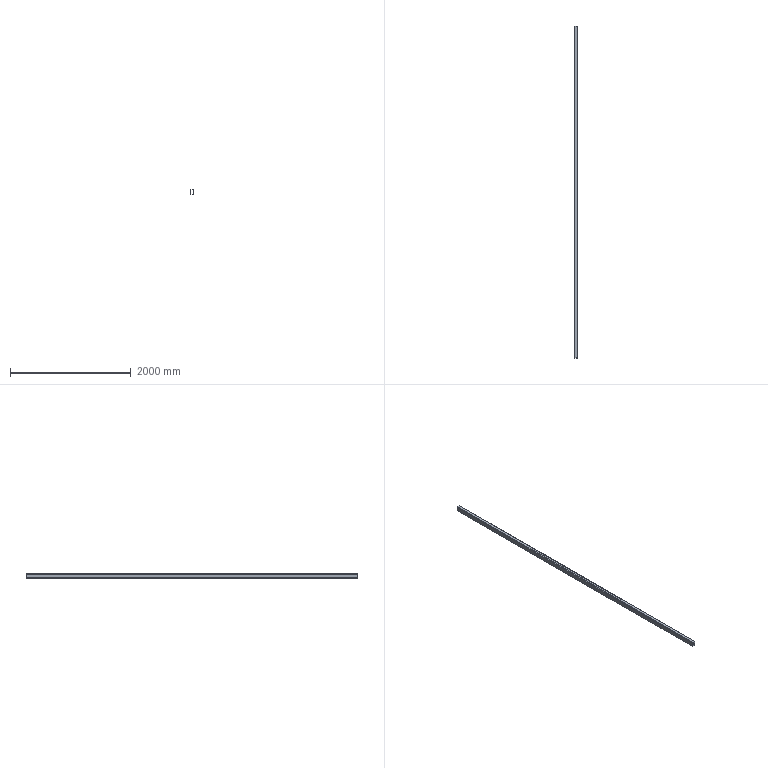Part | SolidWorks | features WeldMemberFeat 1, WeldmentFeature 1 | 1 solid | 18 faces | box 60 x 5500 x 80 mm | volume 6795907 mm3 | plane 10 | cylinder 8 | commonest cylinder face diameters 10 x4 20 x4
STEP:
#1=CARTESIAN_POINT('',(-30.,0.,30.));
#2=VERTEX_POINT('',#1);
#3=CARTESIAN_POINT('',(-20.,0.,40.));
#4=VERTEX_POINT('',#3);
#5=CARTESIAN_POINT('',(-20.,0.,30.));
#6=DIRECTION('',(0.,1.,0.));
#7=DIRECTION('',(0.,0.,1.));
#8=AXIS2_PLACEMENT_3D('',#5,#6,#7);
#9=CIRCLE('',#8,10.);
#10=EDGE_CURVE('',#2,#4,#9,.T.);
#11=ORIENTED_EDGE('',*,*,#10,.T.);
#12=CARTESIAN_POINT('',(-20.,5500.,40.));
#13=VERTEX_POINT('',#12);
#14=CARTESIAN_POINT('',(-20.,5500.,40.));
#15=DIRECTION('',(0.,-1.,0.));
#16=VECTOR('',#15,1000.);
#17=LINE('',#14,#16);
#18=EDGE_CURVE('',#13,#4,#17,.T.);
#19=ORIENTED_EDGE('',*,*,#18,.F.);
#20=CARTESIAN_POINT('',(-30.,5500.,30.));
#21=VERTEX_POINT('',#20);
#22=CARTESIAN_POINT('',(-20.,5500.,30.));
#23=DIRECTION('',(0.,1.,0.));
#24=DIRECTION('',(0.,0.,1.));
#25=AXIS2_PLACEMENT_3D('',#22,#23,#24);
#26=CIRCLE('',#25,10.);
#27=EDGE_CURVE('',#21,#13,#26,.T.);
#28=ORIENTED_EDGE('',*,*,#27,.F.);
#29=CARTESIAN_POINT('',(-30.,5500.,30.));
#30=DIRECTION('',(0.,-1.,0.));
#31=VECTOR('',#30,1000.);
#32=LINE('',#29,#31);
#33=EDGE_CURVE('',#21,#2,#32,.T.);
#34=ORIENTED_EDGE('',*,*,#33,.T.);
#35=EDGE_LOOP('',(#11,#19,#28,#34));
#36=FACE_OUTER_BOUND('',#35,.T.);
#37=CARTESIAN_POINT('',(-20.,5500.,30.));
#38=DIRECTION('',(0.,-1.,0.));
#39=DIRECTION('',(0.,0.,-1.));
#40=AXIS2_PLACEMENT_3D('',#37,#38,#39);
#41=CYLINDRICAL_SURFACE('',#40,10.);
#42=ADVANCED_FACE('',(#36),#41,.T.);
#43=CARTESIAN_POINT('',(20.,0.,40.));
#44=VERTEX_POINT('',#43);
#45=CARTESIAN_POINT('',(-20.,0.,40.));
#46=DIRECTION('',(1.,0.,0.));
#47=VECTOR('',#46,1000.);
#48=LINE('',#45,#47);
#49=EDGE_CURVE('',#4,#44,#48,.T.);
#50=ORIENTED_EDGE('',*,*,#49,.T.);
#51=CARTESIAN_POINT('',(20.,5500.,40.));
#52=VERTEX_POINT('',#51);
#53=CARTESIAN_POINT('',(20.,5500.,40.));
#54=DIRECTION('',(0.,-1.,0.));
#55=VECTOR('',#54,1000.);
#56=LINE('',#53,#55);
#57=EDGE_CURVE('',#52,#44,#56,.T.);
#58=ORIENTED_EDGE('',*,*,#57,.F.);
#59=CARTESIAN_POINT('',(-20.,5500.,40.));
#60=DIRECTION('',(1.,0.,0.));
#61=VECTOR('',#60,1000.);
#62=LINE('',#59,#61);
#63=EDGE_CURVE('',#13,#52,#62,.T.);
#64=ORIENTED_EDGE('',*,*,#63,.F.);
#65=ORIENTED_EDGE('',*,*,#18,.T.);
#66=EDGE_LOOP('',(#50,#58,#64,#65));
#67=FACE_OUTER_BOUND('',#66,.T.);
#68=CARTESIAN_POINT('',(-20.,5500.,40.));
#69=DIRECTION('',(0.,0.,-1.));
#70=DIRECTION('',(-1.,0.,0.));
#71=AXIS2_PLACEMENT_3D('',#68,#69,#70);
#72=PLANE('',#71);
#73=ADVANCED_FACE('',(#67),#72,.F.);
#74=CARTESIAN_POINT('',(30.,0.,30.));
#75=VERTEX_POINT('',#74);
#76=CARTESIAN_POINT('',(20.,0.,30.));
#77=DIRECTION('',(0.,1.,0.));
#78=DIRECTION('',(0.,0.,1.));
#79=AXIS2_PLACEMENT_3D('',#76,#77,#78);
#80=CIRCLE('',#79,10.);
#81=EDGE_CURVE('',#44,#75,#80,.T.);
#82=ORIENTED_EDGE('',*,*,#81,.T.);
#83=CARTESIAN_POINT('',(30.,5500.,30.));
#84=VERTEX_POINT('',#83);
#85=CARTESIAN_POINT('',(30.,5500.,30.));
#86=DIRECTION('',(0.,-1.,0.));
#87=VECTOR('',#86,1000.);
#88=LINE('',#85,#87);
#89=EDGE_CURVE('',#84,#75,#88,.T.);
#90=ORIENTED_EDGE('',*,*,#89,.F.);
#91=CARTESIAN_POINT('',(20.,5500.,30.));
#92=DIRECTION('',(0.,1.,0.));
#93=DIRECTION('',(0.,0.,1.));
#94=AXIS2_PLACEMENT_3D('',#91,#92,#93);
#95=CIRCLE('',#94,10.);
#96=EDGE_CURVE('',#52,#84,#95,.T.);
#97=ORIENTED_EDGE('',*,*,#96,.F.);
#98=ORIENTED_EDGE('',*,*,#57,.T.);
#99=EDGE_LOOP('',(#82,#90,#97,#98));
#100=FACE_OUTER_BOUND('',#99,.T.);
#101=CARTESIAN_POINT('',(20.,5500.,30.));
#102=DIRECTION('',(0.,-1.,0.));
#103=DIRECTION('',(0.,0.,-1.));
#104=AXIS2_PLACEMENT_3D('',#101,#102,#103);
#105=CYLINDRICAL_SURFACE('',#104,10.);
#106=ADVANCED_FACE('',(#100),#105,.T.);
#107=CARTESIAN_POINT('',(30.,0.,-30.));
#108=VERTEX_POINT('',#107);
#109=CARTESIAN_POINT('',(30.,0.,-30.));
#110=DIRECTION('',(0.,0.,-1.));
#111=VECTOR('',#110,1000.);
#112=LINE('',#109,#111);
#113=EDGE_CURVE('',#75,#108,#112,.T.);
#114=ORIENTED_EDGE('',*,*,#113,.T.);
#115=CARTESIAN_POINT('',(30.,5500.,-30.));
#116=VERTEX_POINT('',#115);
#117=CARTESIAN_POINT('',(30.,5500.,-30.));
#118=DIRECTION('',(0.,-1.,0.));
#119=VECTOR('',#118,1000.);
#120=LINE('',#117,#119);
#121=EDGE_CURVE('',#116,#108,#120,.T.);
#122=ORIENTED_EDGE('',*,*,#121,.F.);
#123=CARTESIAN_POINT('',(30.,5500.,-30.));
#124=DIRECTION('',(0.,0.,-1.));
#125=VECTOR('',#124,1000.);
#126=LINE('',#123,#125);
#127=EDGE_CURVE('',#84,#116,#126,.T.);
#128=ORIENTED_EDGE('',*,*,#127,.F.);
#129=ORIENTED_EDGE('',*,*,#89,.T.);
#130=EDGE_LOOP('',(#114,#122,#128,#129));
#131=FACE_OUTER_BOUND('',#130,.T.);
#132=CARTESIAN_POINT('',(30.,5500.,-30.));
#133=DIRECTION('',(-1.,0.,0.));
#134=DIRECTION('',(0.,0.,1.));
#135=AXIS2_PLACEMENT_3D('',#132,#133,#134);
#136=PLANE('',#135);
#137=ADVANCED_FACE('',(#131),#136,.F.);
#138=CARTESIAN_POINT('',(20.,0.,-40.));
#139=VERTEX_POINT('',#138);
#140=CARTESIAN_POINT('',(20.,0.,-30.));
#141=DIRECTION('',(0.,1.,0.));
#142=DIRECTION('',(0.,0.,1.));
#143=AXIS2_PLACEMENT_3D('',#140,#141,#142);
#144=CIRCLE('',#143,10.);
#145=EDGE_CURVE('',#108,#139,#144,.T.);
#146=ORIENTED_EDGE('',*,*,#145,.T.);
#147=CARTESIAN_POINT('',(20.,5500.,-40.));
#148=VERTEX_POINT('',#147);
#149=CARTESIAN_POINT('',(20.,5500.,-40.));
#150=DIRECTION('',(0.,-1.,0.));
#151=VECTOR('',#150,1000.);
#152=LINE('',#149,#151);
#153=EDGE_CURVE('',#148,#139,#152,.T.);
#154=ORIENTED_EDGE('',*,*,#153,.F.);
#155=CARTESIAN_POINT('',(20.,5500.,-30.));
#156=DIRECTION('',(0.,1.,0.));
#157=DIRECTION('',(0.,0.,1.));
#158=AXIS2_PLACEMENT_3D('',#155,#156,#157);
#159=CIRCLE('',#158,10.);
#160=EDGE_CURVE('',#116,#148,#159,.T.);
#161=ORIENTED_EDGE('',*,*,#160,.F.);
#162=ORIENTED_EDGE('',*,*,#121,.T.);
#163=EDGE_LOOP('',(#146,#154,#161,#162));
#164=FACE_OUTER_BOUND('',#163,.T.);
#165=CARTESIAN_POINT('',(20.,5500.,-30.));
#166=DIRECTION('',(0.,-1.,0.));
#167=DIRECTION('',(0.,0.,-1.));
#168=AXIS2_PLACEMENT_3D('',#165,#166,#167);
#169=CYLINDRICAL_SURFACE('',#168,10.);
#170=ADVANCED_FACE('',(#164),#169,.T.);
#171=CARTESIAN_POINT('',(-20.,0.,-40.));
#172=VERTEX_POINT('',#171);
#173=CARTESIAN_POINT('',(20.,0.,-40.));
#174=DIRECTION('',(-1.,0.,0.));
#175=VECTOR('',#174,1000.);
#176=LINE('',#173,#175);
#177=EDGE_CURVE('',#139,#172,#176,.T.);
#178=ORIENTED_EDGE('',*,*,#177,.T.);
#179=CARTESIAN_POINT('',(-20.,5500.,-40.));
#180=VERTEX_POINT('',#179);
#181=CARTESIAN_POINT('',(-20.,5500.,-40.));
#182=DIRECTION('',(0.,-1.,0.));
#183=VECTOR('',#182,1000.);
#184=LINE('',#181,#183);
#185=EDGE_CURVE('',#180,#172,#184,.T.);
#186=ORIENTED_EDGE('',*,*,#185,.F.);
#187=CARTESIAN_POINT('',(20.,5500.,-40.));
#188=DIRECTION('',(-1.,0.,0.));
#189=VECTOR('',#188,1000.);
#190=LINE('',#187,#189);
#191=EDGE_CURVE('',#148,#180,#190,.T.);
#192=ORIENTED_EDGE('',*,*,#191,.F.);
#193=ORIENTED_EDGE('',*,*,#153,.T.);
#194=EDGE_LOOP('',(#178,#186,#192,#193));
#195=FACE_OUTER_BOUND('',#194,.T.);
#196=CARTESIAN_POINT('',(20.,5500.,-40.));
#197=DIRECTION('',(0.,0.,1.));
#198=DIRECTION('',(1.,0.,0.));
#199=AXIS2_PLACEMENT_3D('',#196,#197,#198);
#200=PLANE('',#199);
#201=ADVANCED_FACE('',(#195),#200,.F.);
#202=CARTESIAN_POINT('',(-30.,0.,-30.));
#203=VERTEX_POINT('',#202);
#204=CARTESIAN_POINT('',(-20.,0.,-30.));
#205=DIRECTION('',(0.,1.,0.));
#206=DIRECTION('',(0.,0.,1.));
#207=AXIS2_PLACEMENT_3D('',#204,#205,#206);
#208=CIRCLE('',#207,10.);
#209=EDGE_CURVE('',#172,#203,#208,.T.);
#210=ORIENTED_EDGE('',*,*,#209,.T.);
#211=CARTESIAN_POINT('',(-30.,5500.,-30.));
#212=VERTEX_POINT('',#211);
#213=CARTESIAN_POINT('',(-30.,5500.,-30.));
#214=DIRECTION('',(0.,-1.,0.));
#215=VECTOR('',#214,1000.);
#216=LINE('',#213,#215);
#217=EDGE_CURVE('',#212,#203,#216,.T.);
#218=ORIENTED_EDGE('',*,*,#217,.F.);
#219=CARTESIAN_POINT('',(-20.,5500.,-30.));
#220=DIRECTION('',(0.,1.,0.));
#221=DIRECTION('',(0.,0.,1.));
#222=AXIS2_PLACEMENT_3D('',#219,#220,#221);
#223=CIRCLE('',#222,10.);
#224=EDGE_CURVE('',#180,#212,#223,.T.);
#225=ORIENTED_EDGE('',*,*,#224,.F.);
#226=ORIENTED_EDGE('',*,*,#185,.T.);
#227=EDGE_LOOP('',(#210,#218,#225,#226));
#228=FACE_OUTER_BOUND('',#227,.T.);
#229=CARTESIAN_POINT('',(-20.,5500.,-30.));
#230=DIRECTION('',(0.,-1.,0.));
#231=DIRECTION('',(0.,0.,-1.));
#232=AXIS2_PLACEMENT_3D('',#229,#230,#231);
#233=CYLINDRICAL_SURFACE('',#232,10.);
#234=ADVANCED_FACE('',(#228),#233,.T.);
#235=CARTESIAN_POINT('',(20.,0.,35.));
#236=VERTEX_POINT('',#235);
#237=CARTESIAN_POINT('',(25.,0.,30.));
#238=VERTEX_POINT('',#237);
#239=CARTESIAN_POINT('',(20.,0.,30.));
#240=DIRECTION('',(0.,1.,0.));
#241=DIRECTION('',(0.,0.,1.));
#242=AXIS2_PLACEMENT_3D('',#239,#240,#241);
#243=CIRCLE('',#242,5.);
#244=EDGE_CURVE('',#236,#238,#243,.T.);
#245=ORIENTED_EDGE('',*,*,#244,.F.);
#246=CARTESIAN_POINT('',(20.,5500.,35.));
#247=VERTEX_POINT('',#246);
#248=CARTESIAN_POINT('',(20.,5500.,35.));
#249=DIRECTION('',(0.,-1.,0.));
#250=VECTOR('',#249,1000.);
#251=LINE('',#248,#250);
#252=EDGE_CURVE('',#247,#236,#251,.T.);
#253=ORIENTED_EDGE('',*,*,#252,.F.);
#254=CARTESIAN_POINT('',(25.,5500.,30.));
#255=VERTEX_POINT('',#254);
#256=CARTESIAN_POINT('',(20.,5500.,30.));
#257=DIRECTION('',(0.,1.,0.));
#258=DIRECTION('',(0.,0.,1.));
#259=AXIS2_PLACEMENT_3D('',#256,#257,#258);
#260=CIRCLE('',#259,5.);
#261=EDGE_CURVE('',#247,#255,#260,.T.);
#262=ORIENTED_EDGE('',*,*,#261,.T.);
#263=CARTESIAN_POINT('',(25.,5500.,30.));
#264=DIRECTION('',(0.,-1.,0.));
#265=VECTOR('',#264,1000.);
#266=LINE('',#263,#265);
#267=EDGE_CURVE('',#255,#238,#266,.T.);
#268=ORIENTED_EDGE('',*,*,#267,.T.);
#269=EDGE_LOOP('',(#245,#253,#262,#268));
#270=FACE_OUTER_BOUND('',#269,.T.);
#271=CARTESIAN_POINT('',(20.,5500.,30.));
#272=DIRECTION('',(0.,-1.,0.));
#273=DIRECTION('',(0.,0.,-1.));
#274=AXIS2_PLACEMENT_3D('',#271,#272,#273);
#275=CYLINDRICAL_SURFACE('',#274,5.);
#276=ADVANCED_FACE('',(#270),#275,.F.);
#277=CARTESIAN_POINT('',(-20.,0.,35.));
#278=VERTEX_POINT('',#277);
#279=CARTESIAN_POINT('',(-20.,0.,35.));
#280=DIRECTION('',(1.,0.,0.));
#281=VECTOR('',#280,1000.);
#282=LINE('',#279,#281);
#283=EDGE_CURVE('',#278,#236,#282,.T.);
#284=ORIENTED_EDGE('',*,*,#283,.F.);
#285=CARTESIAN_POINT('',(-20.,5500.,35.));
#286=VERTEX_POINT('',#285);
#287=CARTESIAN_POINT('',(-20.,5500.,35.));
#288=DIRECTION('',(0.,-1.,0.));
#289=VECTOR('',#288,1000.);
#290=LINE('',#287,#289);
#291=EDGE_CURVE('',#286,#278,#290,.T.);
#292=ORIENTED_EDGE('',*,*,#291,.F.);
#293=CARTESIAN_POINT('',(-20.,5500.,35.));
#294=DIRECTION('',(1.,0.,0.));
#295=VECTOR('',#294,1000.);
#296=LINE('',#293,#295);
#297=EDGE_CURVE('',#286,#247,#296,.T.);
#298=ORIENTED_EDGE('',*,*,#297,.T.);
#299=ORIENTED_EDGE('',*,*,#252,.T.);
#300=EDGE_LOOP('',(#284,#292,#298,#299));
#301=FACE_OUTER_BOUND('',#300,.T.);
#302=CARTESIAN_POINT('',(-20.,5500.,35.));
#303=DIRECTION('',(0.,0.,-1.));
#304=DIRECTION('',(-1.,0.,0.));
#305=AXIS2_PLACEMENT_3D('',#302,#303,#304);
#306=PLANE('',#305);
#307=ADVANCED_FACE('',(#301),#306,.T.);
#308=CARTESIAN_POINT('',(-25.,0.,30.));
#309=VERTEX_POINT('',#308);
#310=CARTESIAN_POINT('',(-20.,0.,30.));
#311=DIRECTION('',(0.,1.,0.));
#312=DIRECTION('',(0.,0.,1.));
#313=AXIS2_PLACEMENT_3D('',#310,#311,#312);
#314=CIRCLE('',#313,5.);
#315=EDGE_CURVE('',#309,#278,#314,.T.);
#316=ORIENTED_EDGE('',*,*,#315,.F.);
#317=CARTESIAN_POINT('',(-25.,5500.,30.));
#318=VERTEX_POINT('',#317);
#319=CARTESIAN_POINT('',(-25.,5500.,30.));
#320=DIRECTION('',(0.,-1.,0.));
#321=VECTOR('',#320,1000.);
#322=LINE('',#319,#321);
#323=EDGE_CURVE('',#318,#309,#322,.T.);
#324=ORIENTED_EDGE('',*,*,#323,.F.);
#325=CARTESIAN_POINT('',(-20.,5500.,30.));
#326=DIRECTION('',(0.,1.,0.));
#327=DIRECTION('',(0.,0.,1.));
#328=AXIS2_PLACEMENT_3D('',#325,#326,#327);
#329=CIRCLE('',#328,5.);
#330=EDGE_CURVE('',#318,#286,#329,.T.);
#331=ORIENTED_EDGE('',*,*,#330,.T.);
#332=ORIENTED_EDGE('',*,*,#291,.T.);
#333=EDGE_LOOP('',(#316,#324,#331,#332));
#334=FACE_OUTER_BOUND('',#333,.T.);
#335=CARTESIAN_POINT('',(-20.,5500.,30.));
#336=DIRECTION('',(0.,-1.,0.));
#337=DIRECTION('',(0.,0.,-1.));
#338=AXIS2_PLACEMENT_3D('',#335,#336,#337);
#339=CYLINDRICAL_SURFACE('',#338,5.);
#340=ADVANCED_FACE('',(#334),#339,.F.);
#341=CARTESIAN_POINT('',(-25.,0.,-30.));
#342=VERTEX_POINT('',#341);
#343=CARTESIAN_POINT('',(-25.,0.,30.));
#344=DIRECTION('',(0.,0.,1.));
#345=VECTOR('',#344,1000.);
#346=LINE('',#343,#345);
#347=EDGE_CURVE('',#342,#309,#346,.T.);
#348=ORIENTED_EDGE('',*,*,#347,.F.);
#349=CARTESIAN_POINT('',(-25.,5500.,-30.));
#350=VERTEX_POINT('',#349);
#351=CARTESIAN_POINT('',(-25.,5500.,-30.));
#352=DIRECTION('',(0.,-1.,0.));
#353=VECTOR('',#352,1000.);
#354=LINE('',#351,#353);
#355=EDGE_CURVE('',#350,#342,#354,.T.);
#356=ORIENTED_EDGE('',*,*,#355,.F.);
#357=CARTESIAN_POINT('',(-25.,5500.,30.));
#358=DIRECTION('',(0.,0.,1.));
#359=VECTOR('',#358,1000.);
#360=LINE('',#357,#359);
#361=EDGE_CURVE('',#350,#318,#360,.T.);
#362=ORIENTED_EDGE('',*,*,#361,.T.);
#363=ORIENTED_EDGE('',*,*,#323,.T.);
#364=EDGE_LOOP('',(#348,#356,#362,#363));
#365=FACE_OUTER_BOUND('',#364,.T.);
#366=CARTESIAN_POINT('',(-25.,5500.,30.));
#367=DIRECTION('',(1.,0.,0.));
#368=DIRECTION('',(0.,0.,-1.));
#369=AXIS2_PLACEMENT_3D('',#366,#367,#368);
#370=PLANE('',#369);
#371=ADVANCED_FACE('',(#365),#370,.T.);
#372=CARTESIAN_POINT('',(-20.,0.,-35.));
#373=VERTEX_POINT('',#372);
#374=CARTESIAN_POINT('',(-20.,0.,-30.));
#375=DIRECTION('',(0.,1.,0.));
#376=DIRECTION('',(0.,0.,1.));
#377=AXIS2_PLACEMENT_3D('',#374,#375,#376);
#378=CIRCLE('',#377,5.);
#379=EDGE_CURVE('',#373,#342,#378,.T.);
#380=ORIENTED_EDGE('',*,*,#379,.F.);
#381=CARTESIAN_POINT('',(-20.,5500.,-35.));
#382=VERTEX_POINT('',#381);
#383=CARTESIAN_POINT('',(-20.,5500.,-35.));
#384=DIRECTION('',(0.,-1.,0.));
#385=VECTOR('',#384,1000.);
#386=LINE('',#383,#385);
#387=EDGE_CURVE('',#382,#373,#386,.T.);
#388=ORIENTED_EDGE('',*,*,#387,.F.);
#389=CARTESIAN_POINT('',(-20.,5500.,-30.));
#390=DIRECTION('',(0.,1.,0.));
#391=DIRECTION('',(0.,0.,1.));
#392=AXIS2_PLACEMENT_3D('',#389,#390,#391);
#393=CIRCLE('',#392,5.);
#394=EDGE_CURVE('',#382,#350,#393,.T.);
#395=ORIENTED_EDGE('',*,*,#394,.T.);
#396=ORIENTED_EDGE('',*,*,#355,.T.);
#397=EDGE_LOOP('',(#380,#388,#395,#396));
#398=FACE_OUTER_BOUND('',#397,.T.);
#399=CARTESIAN_POINT('',(-20.,5500.,-30.));
#400=DIRECTION('',(0.,-1.,0.));
#401=DIRECTION('',(0.,0.,-1.));
#402=AXIS2_PLACEMENT_3D('',#399,#400,#401);
#403=CYLINDRICAL_SURFACE('',#402,5.);
#404=ADVANCED_FACE('',(#398),#403,.F.);
#405=CARTESIAN_POINT('',(20.,0.,-35.));
#406=VERTEX_POINT('',#405);
#407=CARTESIAN_POINT('',(20.,0.,-35.));
#408=DIRECTION('',(-1.,0.,0.));
#409=VECTOR('',#408,1000.);
#410=LINE('',#407,#409);
#411=EDGE_CURVE('',#406,#373,#410,.T.);
#412=ORIENTED_EDGE('',*,*,#411,.F.);
#413=CARTESIAN_POINT('',(20.,5500.,-35.));
#414=VERTEX_POINT('',#413);
#415=CARTESIAN_POINT('',(20.,5500.,-35.));
#416=DIRECTION('',(0.,-1.,0.));
#417=VECTOR('',#416,1000.);
#418=LINE('',#415,#417);
#419=EDGE_CURVE('',#414,#406,#418,.T.);
#420=ORIENTED_EDGE('',*,*,#419,.F.);
#421=CARTESIAN_POINT('',(20.,5500.,-35.));
#422=DIRECTION('',(-1.,0.,0.));
#423=VECTOR('',#422,1000.);
#424=LINE('',#421,#423);
#425=EDGE_CURVE('',#414,#382,#424,.T.);
#426=ORIENTED_EDGE('',*,*,#425,.T.);
#427=ORIENTED_EDGE('',*,*,#387,.T.);
#428=EDGE_LOOP('',(#412,#420,#426,#427));
#429=FACE_OUTER_BOUND('',#428,.T.);
#430=CARTESIAN_POINT('',(20.,5500.,-35.));
#431=DIRECTION('',(0.,0.,1.));
#432=DIRECTION('',(1.,0.,0.));
#433=AXIS2_PLACEMENT_3D('',#430,#431,#432);
#434=PLANE('',#433);
#435=ADVANCED_FACE('',(#429),#434,.T.);
#436=CARTESIAN_POINT('',(25.,0.,-30.));
#437=VERTEX_POINT('',#436);
#438=CARTESIAN_POINT('',(20.,0.,-30.));
#439=DIRECTION('',(0.,1.,0.));
#440=DIRECTION('',(0.,0.,1.));
#441=AXIS2_PLACEMENT_3D('',#438,#439,#440);
#442=CIRCLE('',#441,5.);
#443=EDGE_CURVE('',#437,#406,#442,.T.);
#444=ORIENTED_EDGE('',*,*,#443,.F.);
#445=CARTESIAN_POINT('',(25.,5500.,-30.));
#446=VERTEX_POINT('',#445);
#447=CARTESIAN_POINT('',(25.,5500.,-30.));
#448=DIRECTION('',(0.,-1.,0.));
#449=VECTOR('',#448,1000.);
#450=LINE('',#447,#449);
#451=EDGE_CURVE('',#446,#437,#450,.T.);
#452=ORIENTED_EDGE('',*,*,#451,.F.);
#453=CARTESIAN_POINT('',(20.,5500.,-30.));
#454=DIRECTION('',(0.,1.,0.));
#455=DIRECTION('',(0.,0.,1.));
#456=AXIS2_PLACEMENT_3D('',#453,#454,#455);
#457=CIRCLE('',#456,5.);
#458=EDGE_CURVE('',#446,#414,#457,.T.);
#459=ORIENTED_EDGE('',*,*,#458,.T.);
#460=ORIENTED_EDGE('',*,*,#419,.T.);
#461=EDGE_LOOP('',(#444,#452,#459,#460));
#462=FACE_OUTER_BOUND('',#461,.T.);
#463=CARTESIAN_POINT('',(20.,5500.,-30.));
#464=DIRECTION('',(0.,-1.,0.));
#465=DIRECTION('',(0.,0.,-1.));
#466=AXIS2_PLACEMENT_3D('',#463,#464,#465);
#467=CYLINDRICAL_SURFACE('',#466,5.);
#468=ADVANCED_FACE('',(#462),#467,.F.);
#469=CARTESIAN_POINT('',(25.,0.,-30.));
#470=DIRECTION('',(0.,0.,-1.));
#471=VECTOR('',#470,1000.);
#472=LINE('',#469,#471);
#473=EDGE_CURVE('',#238,#437,#472,.T.);
#474=ORIENTED_EDGE('',*,*,#473,.F.);
#475=ORIENTED_EDGE('',*,*,#267,.F.);
#476=CARTESIAN_POINT('',(25.,5500.,-30.));
#477=DIRECTION('',(0.,0.,-1.));
#478=VECTOR('',#477,1000.);
#479=LINE('',#476,#478);
#480=EDGE_CURVE('',#255,#446,#479,.T.);
#481=ORIENTED_EDGE('',*,*,#480,.T.);
#482=ORIENTED_EDGE('',*,*,#451,.T.);
#483=EDGE_LOOP('',(#474,#475,#481,#482));
#484=FACE_OUTER_BOUND('',#483,.T.);
#485=CARTESIAN_POINT('',(25.,5500.,-30.));
#486=DIRECTION('',(-1.,0.,0.));
#487=DIRECTION('',(0.,0.,1.));
#488=AXIS2_PLACEMENT_3D('',#485,#486,#487);
#489=PLANE('',#488);
#490=ADVANCED_FACE('',(#484),#489,.T.);
#491=CARTESIAN_POINT('',(-30.,0.,30.));
#492=DIRECTION('',(0.,0.,1.));
#493=VECTOR('',#492,1000.);
#494=LINE('',#491,#493);
#495=EDGE_CURVE('',#203,#2,#494,.T.);
#496=ORIENTED_EDGE('',*,*,#495,.T.);
#497=ORIENTED_EDGE('',*,*,#33,.F.);
#498=CARTESIAN_POINT('',(-30.,5500.,30.));
#499=DIRECTION('',(0.,0.,1.));
#500=VECTOR('',#499,1000.);
#501=LINE('',#498,#500);
#502=EDGE_CURVE('',#212,#21,#501,.T.);
#503=ORIENTED_EDGE('',*,*,#502,.F.);
#504=ORIENTED_EDGE('',*,*,#217,.T.);
#505=EDGE_LOOP('',(#496,#497,#503,#504));
#506=FACE_OUTER_BOUND('',#505,.T.);
#507=CARTESIAN_POINT('',(-30.,5500.,30.));
#508=DIRECTION('',(1.,0.,0.));
#509=DIRECTION('',(0.,0.,-1.));
#510=AXIS2_PLACEMENT_3D('',#507,#508,#509);
#511=PLANE('',#510);
#512=ADVANCED_FACE('',(#506),#511,.F.);
#513=ORIENTED_EDGE('',*,*,#261,.F.);
#514=ORIENTED_EDGE('',*,*,#297,.F.);
#515=ORIENTED_EDGE('',*,*,#330,.F.);
#516=ORIENTED_EDGE('',*,*,#361,.F.);
#517=ORIENTED_EDGE('',*,*,#394,.F.);
#518=ORIENTED_EDGE('',*,*,#425,.F.);
#519=ORIENTED_EDGE('',*,*,#458,.F.);
#520=ORIENTED_EDGE('',*,*,#480,.F.);
#521=EDGE_LOOP('',(#513,#514,#515,#516,#517,#518,#519,#520));
#522=FACE_BOUND('',#521,.T.);
#523=ORIENTED_EDGE('',*,*,#27,.T.);
#524=ORIENTED_EDGE('',*,*,#63,.T.);
#525=ORIENTED_EDGE('',*,*,#96,.T.);
#526=ORIENTED_EDGE('',*,*,#127,.T.);
#527=ORIENTED_EDGE('',*,*,#160,.T.);
#528=ORIENTED_EDGE('',*,*,#191,.T.);
#529=ORIENTED_EDGE('',*,*,#224,.T.);
#530=ORIENTED_EDGE('',*,*,#502,.T.);
#531=EDGE_LOOP('',(#523,#524,#525,#526,#527,#528,#529,#530));
#532=FACE_OUTER_BOUND('',#531,.T.);
#533=CARTESIAN_POINT('',(-20.,5500.,30.));
#534=DIRECTION('',(0.,1.,0.));
#535=DIRECTION('',(0.,0.,1.));
#536=AXIS2_PLACEMENT_3D('',#533,#534,#535);
#537=PLANE('',#536);
#538=ADVANCED_FACE('',(#522,#532),#537,.T.);
#539=ORIENTED_EDGE('',*,*,#244,.T.);
#540=ORIENTED_EDGE('',*,*,#473,.T.);
#541=ORIENTED_EDGE('',*,*,#443,.T.);
#542=ORIENTED_EDGE('',*,*,#411,.T.);
#543=ORIENTED_EDGE('',*,*,#379,.T.);
#544=ORIENTED_EDGE('',*,*,#347,.T.);
#545=ORIENTED_EDGE('',*,*,#315,.T.);
#546=ORIENTED_EDGE('',*,*,#283,.T.);
#547=EDGE_LOOP('',(#539,#540,#541,#542,#543,#544,#545,#546));
#548=FACE_BOUND('',#547,.T.);
#549=ORIENTED_EDGE('',*,*,#10,.F.);
#550=ORIENTED_EDGE('',*,*,#495,.F.);
#551=ORIENTED_EDGE('',*,*,#209,.F.);
#552=ORIENTED_EDGE('',*,*,#177,.F.);
#553=ORIENTED_EDGE('',*,*,#145,.F.);
#554=ORIENTED_EDGE('',*,*,#113,.F.);
#555=ORIENTED_EDGE('',*,*,#81,.F.);
#556=ORIENTED_EDGE('',*,*,#49,.F.);
#557=EDGE_LOOP('',(#549,#550,#551,#552,#553,#554,#555,#556));
#558=FACE_OUTER_BOUND('',#557,.T.);
#559=CARTESIAN_POINT('',(-20.,0.,30.));
#560=DIRECTION('',(0.,1.,0.));
#561=DIRECTION('',(0.,0.,1.));
#562=AXIS2_PLACEMENT_3D('',#559,#560,#561);
#563=PLANE('',#562);
#564=ADVANCED_FACE('',(#548,#558),#563,.F.);
#565=CLOSED_SHELL('',(#42,#73,#106,#137,#170,#201,#234,#276,#307,#340,#371,#404,#435,#468,#490,#512,#538,#564));
#566=MANIFOLD_SOLID_BREP('',#565);
#567=CARTESIAN_POINT('',(0.,0.,0.));
#568=DIRECTION('',(0.,0.,1.));
#569=DIRECTION('',(1.,0.,0.));
#570=AXIS2_PLACEMENT_3D('',#567,#568,#569);
#571=(LENGTH_UNIT()NAMED_UNIT(*)SI_UNIT(.MILLI.,.METRE.));
#572=UNCERTAINTY_MEASURE_WITH_UNIT(LENGTH_MEASURE(0.00001),#571,'','');
#573=(NAMED_UNIT(*)PLANE_ANGLE_UNIT()SI_UNIT($,.RADIAN.));
#574=(NAMED_UNIT(*)SI_UNIT($,.STERADIAN.)SOLID_ANGLE_UNIT());
#575=(GEOMETRIC_REPRESENTATION_CONTEXT(3)GLOBAL_UNCERTAINTY_ASSIGNED_CONTEXT((#572))GLOBAL_UNIT_ASSIGNED_CONTEXT((#571,#573,#574))REPRESENTATION_CONTEXT('',''));
#576=ADVANCED_BREP_SHAPE_REPRESENTATION('',(#566,#570),#575);